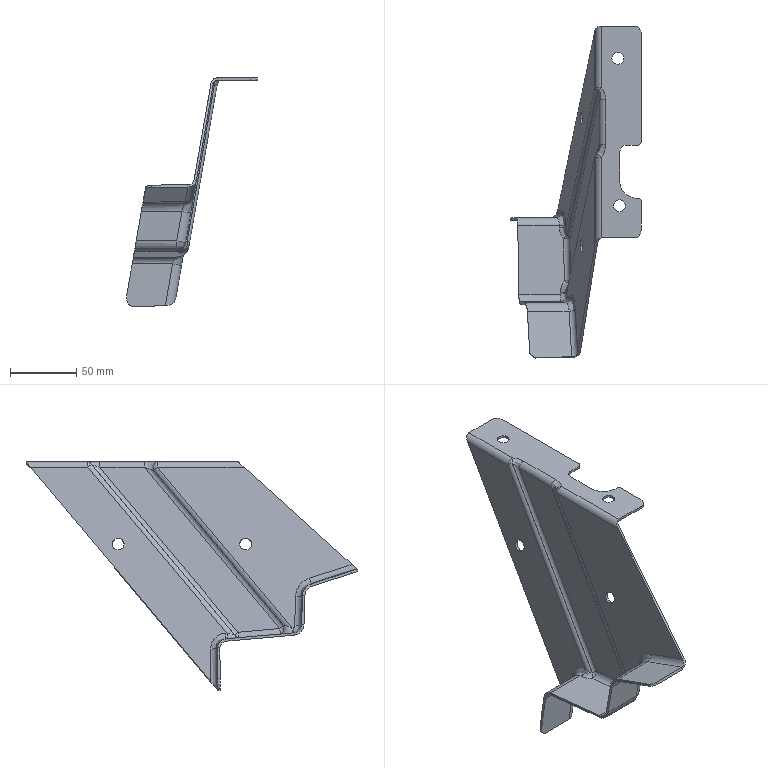Part | 1 solid | 120 faces | box 98.458 x 249.655 x 171.852 mm | volume 56525 mm3 | cylinder 48 | spline 36 | plane 24 | sphere 8 | other 4 | commonest cylinder face diameters 10 x19 13.6 x11 6.4 x7 9 x4 16 x2 5 x1